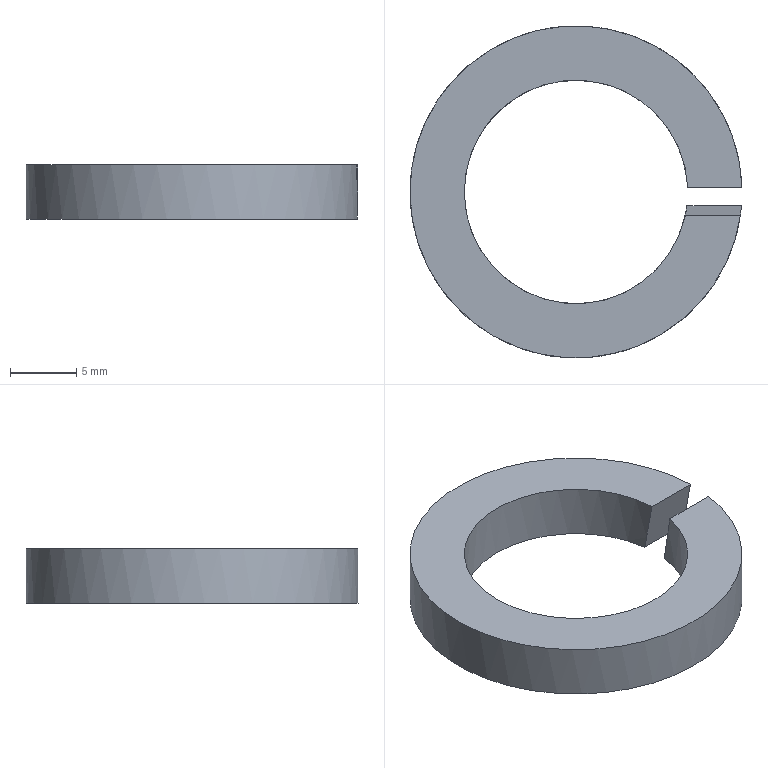Part | NX | features DATUM_CSYS 2, SKETCH 2, EXTRUDE 1, LINE 1, META 1, SWP104 1 | 1 solid | 6 faces | box 25.096 x 25.1 x 4.1 mm | volume 1074 mm3 | plane 4 | cylinder 2 | commonest cylinder face diameters 16.9 x1 25.1 x1
STEP:
#1=CARTESIAN_POINT('',(12.507,-1.041,0.));
#2=VERTEX_POINT('',#1);
#3=CARTESIAN_POINT('',(12.507,1.041,0.));
#4=VERTEX_POINT('',#3);
#5=CARTESIAN_POINT('',(0.,0.,0.));
#6=DIRECTION('',(0.,0.,-1.));
#7=DIRECTION('',(-1.,0.,0.));
#8=AXIS2_PLACEMENT_3D('',#5,#6,#7);
#9=CIRCLE('',#8,12.55);
#10=EDGE_CURVE('',#2,#4,#9,.T.);
#11=ORIENTED_EDGE('',*,*,#10,.F.);
#12=CARTESIAN_POINT('',(12.425,-1.764,4.1));
#13=VERTEX_POINT('',#12);
#14=CARTESIAN_POINT('',(0.,0.,-5.903));
#15=DIRECTION('',(0.,0.9848,0.1736));
#16=DIRECTION('',(0.,0.1736,-0.9848));
#17=AXIS2_PLACEMENT_3D('',#14,#15,#16);
#18=ELLIPSE('',#17,72.273,12.55);
#19=EDGE_CURVE('',#2,#13,#18,.F.);
#20=ORIENTED_EDGE('',*,*,#19,.T.);
#21=CARTESIAN_POINT('',(12.546,0.3179,4.1));
#22=VERTEX_POINT('',#21);
#23=CARTESIAN_POINT('',(0.,0.,4.1));
#24=DIRECTION('',(0.,0.,-1.));
#25=DIRECTION('',(-1.,0.,0.));
#26=AXIS2_PLACEMENT_3D('',#23,#24,#25);
#27=CIRCLE('',#26,12.55);
#28=EDGE_CURVE('',#13,#22,#27,.T.);
#29=ORIENTED_EDGE('',*,*,#28,.T.);
#30=CARTESIAN_POINT('',(0.,0.,5.903));
#31=DIRECTION('',(0.,-0.9848,-0.1736));
#32=DIRECTION('',(0.,0.1736,-0.9848));
#33=AXIS2_PLACEMENT_3D('',#30,#31,#32);
#34=ELLIPSE('',#33,72.273,12.55);
#35=EDGE_CURVE('',#22,#4,#34,.F.);
#36=ORIENTED_EDGE('',*,*,#35,.T.);
#37=EDGE_LOOP('',(#11,#20,#29,#36));
#38=FACE_BOUND('',#37,.T.);
#39=CARTESIAN_POINT('',(0.,0.,0.));
#40=DIRECTION('',(0.,0.,-1.));
#41=DIRECTION('',(-1.,0.,0.));
#42=AXIS2_PLACEMENT_3D('',#39,#40,#41);
#43=CYLINDRICAL_SURFACE('',#42,12.55);
#44=ADVANCED_FACE('',(#38),#43,.T.);
#45=ORIENTED_EDGE('',*,*,#28,.F.);
#46=CARTESIAN_POINT('',(8.264,-1.764,4.1));
#47=VERTEX_POINT('',#46);
#48=CARTESIAN_POINT('',(0.,-1.764,4.1));
#49=DIRECTION('',(-1.,0.,0.));
#50=VECTOR('',#49,1000.);
#51=LINE('',#48,#50);
#52=EDGE_CURVE('',#13,#47,#51,.T.);
#53=ORIENTED_EDGE('',*,*,#52,.T.);
#54=CARTESIAN_POINT('',(8.444,0.3179,4.1));
#55=VERTEX_POINT('',#54);
#56=CARTESIAN_POINT('',(0.,0.,4.1));
#57=DIRECTION('',(0.,0.,-1.));
#58=DIRECTION('',(-1.,0.,0.));
#59=AXIS2_PLACEMENT_3D('',#56,#57,#58);
#60=CIRCLE('',#59,8.45);
#61=EDGE_CURVE('',#47,#55,#60,.T.);
#62=ORIENTED_EDGE('',*,*,#61,.T.);
#63=CARTESIAN_POINT('',(0.,0.3179,4.1));
#64=DIRECTION('',(1.,0.,0.));
#65=VECTOR('',#64,1000.);
#66=LINE('',#63,#65);
#67=EDGE_CURVE('',#55,#22,#66,.T.);
#68=ORIENTED_EDGE('',*,*,#67,.T.);
#69=EDGE_LOOP('',(#45,#53,#62,#68));
#70=FACE_BOUND('',#69,.T.);
#71=CARTESIAN_POINT('',(0.,12.55,4.1));
#72=DIRECTION('',(0.,0.,1.));
#73=DIRECTION('',(1.,0.,0.));
#74=AXIS2_PLACEMENT_3D('',#71,#72,#73);
#75=PLANE('',#74);
#76=ADVANCED_FACE('',(#70),#75,.T.);
#77=ORIENTED_EDGE('',*,*,#61,.F.);
#78=CARTESIAN_POINT('',(8.386,-1.041,0.));
#79=VERTEX_POINT('',#78);
#80=CARTESIAN_POINT('',(0.,0.,-5.903));
#81=DIRECTION('',(0.,0.9848,0.1736));
#82=DIRECTION('',(0.,0.1736,-0.9848));
#83=AXIS2_PLACEMENT_3D('',#80,#81,#82);
#84=ELLIPSE('',#83,48.662,8.45);
#85=EDGE_CURVE('',#47,#79,#84,.T.);
#86=ORIENTED_EDGE('',*,*,#85,.T.);
#87=CARTESIAN_POINT('',(8.386,1.041,0.));
#88=VERTEX_POINT('',#87);
#89=CARTESIAN_POINT('',(0.,0.,0.));
#90=DIRECTION('',(0.,0.,-1.));
#91=DIRECTION('',(-1.,0.,0.));
#92=AXIS2_PLACEMENT_3D('',#89,#90,#91);
#93=CIRCLE('',#92,8.45);
#94=EDGE_CURVE('',#79,#88,#93,.T.);
#95=ORIENTED_EDGE('',*,*,#94,.T.);
#96=CARTESIAN_POINT('',(0.,0.,5.903));
#97=DIRECTION('',(0.,-0.9848,-0.1736));
#98=DIRECTION('',(0.,0.1736,-0.9848));
#99=AXIS2_PLACEMENT_3D('',#96,#97,#98);
#100=ELLIPSE('',#99,48.662,8.45);
#101=EDGE_CURVE('',#88,#55,#100,.T.);
#102=ORIENTED_EDGE('',*,*,#101,.T.);
#103=EDGE_LOOP('',(#77,#86,#95,#102));
#104=FACE_BOUND('',#103,.T.);
#105=CARTESIAN_POINT('',(0.,0.,0.));
#106=DIRECTION('',(0.,0.,-1.));
#107=DIRECTION('',(-1.,0.,0.));
#108=AXIS2_PLACEMENT_3D('',#105,#106,#107);
#109=CYLINDRICAL_SURFACE('',#108,8.45);
#110=ADVANCED_FACE('',(#104),#109,.F.);
#111=ORIENTED_EDGE('',*,*,#94,.F.);
#112=CARTESIAN_POINT('',(0.,-1.041,0.));
#113=DIRECTION('',(1.,0.,0.));
#114=VECTOR('',#113,1000.);
#115=LINE('',#112,#114);
#116=EDGE_CURVE('',#79,#2,#115,.T.);
#117=ORIENTED_EDGE('',*,*,#116,.T.);
#118=ORIENTED_EDGE('',*,*,#10,.T.);
#119=CARTESIAN_POINT('',(0.,1.041,0.));
#120=DIRECTION('',(-1.,0.,0.));
#121=VECTOR('',#120,1000.);
#122=LINE('',#119,#121);
#123=EDGE_CURVE('',#4,#88,#122,.T.);
#124=ORIENTED_EDGE('',*,*,#123,.T.);
#125=EDGE_LOOP('',(#111,#117,#118,#124));
#126=FACE_BOUND('',#125,.T.);
#127=CARTESIAN_POINT('',(0.,8.45,0.));
#128=DIRECTION('',(0.,0.,-1.));
#129=DIRECTION('',(-1.,0.,0.));
#130=AXIS2_PLACEMENT_3D('',#127,#128,#129);
#131=PLANE('',#130);
#132=ADVANCED_FACE('',(#126),#131,.T.);
#133=ORIENTED_EDGE('',*,*,#67,.F.);
#134=ORIENTED_EDGE('',*,*,#101,.F.);
#135=ORIENTED_EDGE('',*,*,#123,.F.);
#136=ORIENTED_EDGE('',*,*,#35,.F.);
#137=EDGE_LOOP('',(#133,#134,#135,#136));
#138=FACE_BOUND('',#137,.T.);
#139=CARTESIAN_POINT('',(18.825,2.077,-5.879));
#140=DIRECTION('',(0.,-0.9848,-0.1736));
#141=DIRECTION('',(0.,0.1736,-0.9848));
#142=AXIS2_PLACEMENT_3D('',#139,#140,#141);
#143=PLANE('',#142);
#144=ADVANCED_FACE('',(#138),#143,.T.);
#145=ORIENTED_EDGE('',*,*,#116,.F.);
#146=ORIENTED_EDGE('',*,*,#85,.F.);
#147=ORIENTED_EDGE('',*,*,#52,.F.);
#148=ORIENTED_EDGE('',*,*,#19,.F.);
#149=EDGE_LOOP('',(#145,#146,#147,#148));
#150=FACE_BOUND('',#149,.T.);
#151=CARTESIAN_POINT('',(18.825,-2.077,5.879));
#152=DIRECTION('',(0.,0.9848,0.1736));
#153=DIRECTION('',(0.,-0.1736,0.9848));
#154=AXIS2_PLACEMENT_3D('',#151,#152,#153);
#155=PLANE('',#154);
#156=ADVANCED_FACE('',(#150),#155,.T.);
#157=CLOSED_SHELL('',(#44,#76,#110,#132,#144,#156));
#158=MANIFOLD_SOLID_BREP('',#157);
#159=(LENGTH_UNIT()NAMED_UNIT(*)SI_UNIT(.MILLI.,.METRE.));
#160=UNCERTAINTY_MEASURE_WITH_UNIT(LENGTH_MEASURE(0.00001),#159,'','');
#161=(NAMED_UNIT(*)PLANE_ANGLE_UNIT()SI_UNIT($,.RADIAN.));
#162=(NAMED_UNIT(*)SI_UNIT($,.STERADIAN.)SOLID_ANGLE_UNIT());
#163=(GEOMETRIC_REPRESENTATION_CONTEXT(3)GLOBAL_UNCERTAINTY_ASSIGNED_CONTEXT((#160))GLOBAL_UNIT_ASSIGNED_CONTEXT((#159,#161,#162))REPRESENTATION_CONTEXT('',''));
#164=ADVANCED_BREP_SHAPE_REPRESENTATION('',(#158),#163);